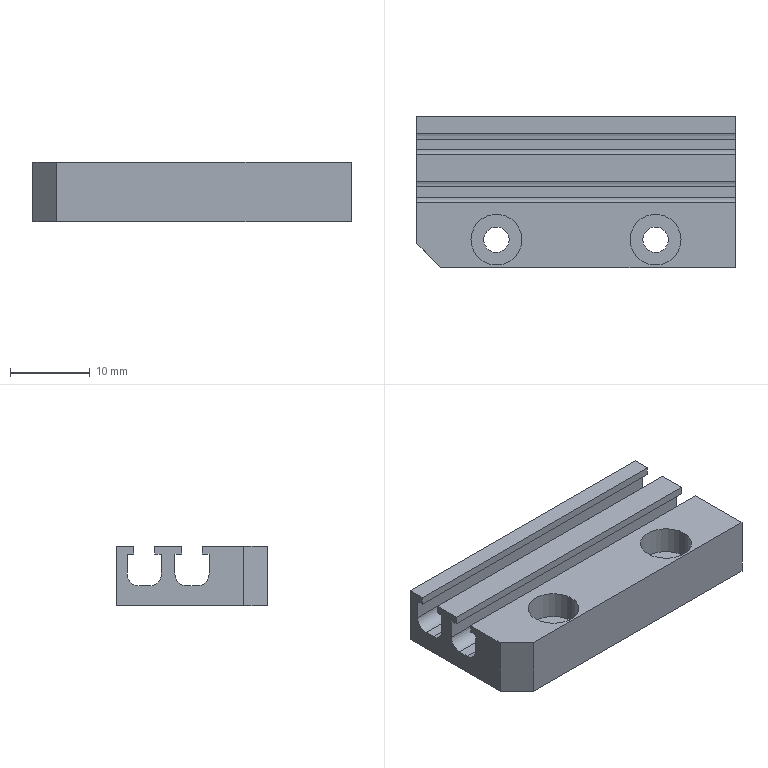Part | NX | 1 solid | 37 faces | box 40 x 19 x 7.5 mm | volume 3870 mm3 | plane 25 | cylinder 12 | commonest cylinder face diameters 3 x4 3.2 x4 6.4 x4
STEP:
#1=CARTESIAN_POINT('',(-20.,16.8,0.));
#2=VERTEX_POINT('',#1);
#3=CARTESIAN_POINT('',(-20.,19.,0.));
#4=VERTEX_POINT('',#3);
#5=CARTESIAN_POINT('',(-20.,16.8,0.));
#6=DIRECTION('',(0.,1.,0.));
#7=VECTOR('',#6,1000.);
#8=LINE('',#5,#7);
#9=EDGE_CURVE('',#2,#4,#8,.T.);
#10=ORIENTED_EDGE('',*,*,#9,.T.);
#11=CARTESIAN_POINT('',(-20.,19.,-7.5));
#12=VERTEX_POINT('',#11);
#13=CARTESIAN_POINT('',(-20.,19.,0.));
#14=DIRECTION('',(0.,0.,-1.));
#15=VECTOR('',#14,1000.);
#16=LINE('',#13,#15);
#17=EDGE_CURVE('',#4,#12,#16,.T.);
#18=ORIENTED_EDGE('',*,*,#17,.T.);
#19=CARTESIAN_POINT('',(-20.,3.,-7.5));
#20=VERTEX_POINT('',#19);
#21=CARTESIAN_POINT('',(-20.,19.,-7.5));
#22=DIRECTION('',(0.,-1.,0.));
#23=VECTOR('',#22,1000.);
#24=LINE('',#21,#23);
#25=EDGE_CURVE('',#12,#20,#24,.T.);
#26=ORIENTED_EDGE('',*,*,#25,.T.);
#27=CARTESIAN_POINT('',(-20.,3.,0.));
#28=VERTEX_POINT('',#27);
#29=CARTESIAN_POINT('',(-20.,3.,-7.5));
#30=DIRECTION('',(0.,0.,1.));
#31=VECTOR('',#30,1000.);
#32=LINE('',#29,#31);
#33=EDGE_CURVE('',#20,#28,#32,.T.);
#34=ORIENTED_EDGE('',*,*,#33,.T.);
#35=CARTESIAN_POINT('',(-20.,8.2,0.));
#36=VERTEX_POINT('',#35);
#37=CARTESIAN_POINT('',(-20.,3.,0.));
#38=DIRECTION('',(0.,1.,0.));
#39=VECTOR('',#38,1000.);
#40=LINE('',#37,#39);
#41=EDGE_CURVE('',#28,#36,#40,.T.);
#42=ORIENTED_EDGE('',*,*,#41,.T.);
#43=CARTESIAN_POINT('',(-20.,8.2,-1.));
#44=VERTEX_POINT('',#43);
#45=CARTESIAN_POINT('',(-20.,8.2,0.));
#46=DIRECTION('',(0.,0.,-1.));
#47=VECTOR('',#46,1000.);
#48=LINE('',#45,#47);
#49=EDGE_CURVE('',#36,#44,#48,.T.);
#50=ORIENTED_EDGE('',*,*,#49,.T.);
#51=CARTESIAN_POINT('',(-20.,7.35,-1.));
#52=VERTEX_POINT('',#51);
#53=CARTESIAN_POINT('',(-20.,8.2,-1.));
#54=DIRECTION('',(0.,-1.,0.));
#55=VECTOR('',#54,1000.);
#56=LINE('',#53,#55);
#57=EDGE_CURVE('',#44,#52,#56,.T.);
#58=ORIENTED_EDGE('',*,*,#57,.T.);
#59=CARTESIAN_POINT('',(-20.,7.35,-3.5));
#60=VERTEX_POINT('',#59);
#61=CARTESIAN_POINT('',(-20.,7.35,-1.));
#62=DIRECTION('',(0.,0.,-1.));
#63=VECTOR('',#62,1000.);
#64=LINE('',#61,#63);
#65=EDGE_CURVE('',#52,#60,#64,.T.);
#66=ORIENTED_EDGE('',*,*,#65,.T.);
#67=CARTESIAN_POINT('',(-20.,8.85,-5.));
#68=VERTEX_POINT('',#67);
#69=CARTESIAN_POINT('',(-20.,8.85,-3.5));
#70=DIRECTION('',(-1.,0.,0.));
#71=DIRECTION('',(0.,0.,-1.));
#72=AXIS2_PLACEMENT_3D('',#69,#70,#71);
#73=CIRCLE('',#72,1.5);
#74=EDGE_CURVE('',#68,#60,#73,.T.);
#75=ORIENTED_EDGE('',*,*,#74,.F.);
#76=CARTESIAN_POINT('',(-20.,10.15,-5.));
#77=VERTEX_POINT('',#76);
#78=CARTESIAN_POINT('',(-20.,8.85,-5.));
#79=DIRECTION('',(0.,1.,0.));
#80=VECTOR('',#79,1000.);
#81=LINE('',#78,#80);
#82=EDGE_CURVE('',#68,#77,#81,.T.);
#83=ORIENTED_EDGE('',*,*,#82,.T.);
#84=CARTESIAN_POINT('',(-20.,11.65,-3.5));
#85=VERTEX_POINT('',#84);
#86=CARTESIAN_POINT('',(-20.,10.15,-3.5));
#87=DIRECTION('',(-1.,0.,0.));
#88=DIRECTION('',(0.,1.,0.));
#89=AXIS2_PLACEMENT_3D('',#86,#87,#88);
#90=CIRCLE('',#89,1.5);
#91=EDGE_CURVE('',#85,#77,#90,.T.);
#92=ORIENTED_EDGE('',*,*,#91,.F.);
#93=CARTESIAN_POINT('',(-20.,11.65,-1.));
#94=VERTEX_POINT('',#93);
#95=CARTESIAN_POINT('',(-20.,11.65,-3.5));
#96=DIRECTION('',(0.,0.,1.));
#97=VECTOR('',#96,1000.);
#98=LINE('',#95,#97);
#99=EDGE_CURVE('',#85,#94,#98,.T.);
#100=ORIENTED_EDGE('',*,*,#99,.T.);
#101=CARTESIAN_POINT('',(-20.,10.8,-1.));
#102=VERTEX_POINT('',#101);
#103=CARTESIAN_POINT('',(-20.,11.65,-1.));
#104=DIRECTION('',(0.,-1.,0.));
#105=VECTOR('',#104,1000.);
#106=LINE('',#103,#105);
#107=EDGE_CURVE('',#94,#102,#106,.T.);
#108=ORIENTED_EDGE('',*,*,#107,.T.);
#109=CARTESIAN_POINT('',(-20.,10.8,0.));
#110=VERTEX_POINT('',#109);
#111=CARTESIAN_POINT('',(-20.,10.8,-1.));
#112=DIRECTION('',(0.,0.,1.));
#113=VECTOR('',#112,1000.);
#114=LINE('',#111,#113);
#115=EDGE_CURVE('',#102,#110,#114,.T.);
#116=ORIENTED_EDGE('',*,*,#115,.T.);
#117=CARTESIAN_POINT('',(-20.,14.2,0.));
#118=VERTEX_POINT('',#117);
#119=CARTESIAN_POINT('',(-20.,10.8,0.));
#120=DIRECTION('',(0.,1.,0.));
#121=VECTOR('',#120,1000.);
#122=LINE('',#119,#121);
#123=EDGE_CURVE('',#110,#118,#122,.T.);
#124=ORIENTED_EDGE('',*,*,#123,.T.);
#125=CARTESIAN_POINT('',(-20.,14.2,-1.));
#126=VERTEX_POINT('',#125);
#127=CARTESIAN_POINT('',(-20.,14.2,0.));
#128=DIRECTION('',(0.,0.,-1.));
#129=VECTOR('',#128,1000.);
#130=LINE('',#127,#129);
#131=EDGE_CURVE('',#118,#126,#130,.T.);
#132=ORIENTED_EDGE('',*,*,#131,.T.);
#133=CARTESIAN_POINT('',(-20.,13.35,-1.));
#134=VERTEX_POINT('',#133);
#135=CARTESIAN_POINT('',(-20.,14.2,-1.));
#136=DIRECTION('',(0.,-1.,0.));
#137=VECTOR('',#136,1000.);
#138=LINE('',#135,#137);
#139=EDGE_CURVE('',#126,#134,#138,.T.);
#140=ORIENTED_EDGE('',*,*,#139,.T.);
#141=CARTESIAN_POINT('',(-20.,13.35,-3.5));
#142=VERTEX_POINT('',#141);
#143=CARTESIAN_POINT('',(-20.,13.35,-1.));
#144=DIRECTION('',(0.,0.,-1.));
#145=VECTOR('',#144,1000.);
#146=LINE('',#143,#145);
#147=EDGE_CURVE('',#134,#142,#146,.T.);
#148=ORIENTED_EDGE('',*,*,#147,.T.);
#149=CARTESIAN_POINT('',(-20.,14.85,-5.));
#150=VERTEX_POINT('',#149);
#151=CARTESIAN_POINT('',(-20.,14.85,-3.5));
#152=DIRECTION('',(-1.,0.,0.));
#153=DIRECTION('',(0.,0.,-1.));
#154=AXIS2_PLACEMENT_3D('',#151,#152,#153);
#155=CIRCLE('',#154,1.5);
#156=EDGE_CURVE('',#150,#142,#155,.T.);
#157=ORIENTED_EDGE('',*,*,#156,.F.);
#158=CARTESIAN_POINT('',(-20.,16.15,-5.));
#159=VERTEX_POINT('',#158);
#160=CARTESIAN_POINT('',(-20.,14.85,-5.));
#161=DIRECTION('',(0.,1.,0.));
#162=VECTOR('',#161,1000.);
#163=LINE('',#160,#162);
#164=EDGE_CURVE('',#150,#159,#163,.T.);
#165=ORIENTED_EDGE('',*,*,#164,.T.);
#166=CARTESIAN_POINT('',(-20.,17.65,-3.5));
#167=VERTEX_POINT('',#166);
#168=CARTESIAN_POINT('',(-20.,16.15,-3.5));
#169=DIRECTION('',(-1.,0.,0.));
#170=DIRECTION('',(0.,1.,0.));
#171=AXIS2_PLACEMENT_3D('',#168,#169,#170);
#172=CIRCLE('',#171,1.5);
#173=EDGE_CURVE('',#167,#159,#172,.T.);
#174=ORIENTED_EDGE('',*,*,#173,.F.);
#175=CARTESIAN_POINT('',(-20.,17.65,-1.));
#176=VERTEX_POINT('',#175);
#177=CARTESIAN_POINT('',(-20.,17.65,-3.5));
#178=DIRECTION('',(0.,0.,1.));
#179=VECTOR('',#178,1000.);
#180=LINE('',#177,#179);
#181=EDGE_CURVE('',#167,#176,#180,.T.);
#182=ORIENTED_EDGE('',*,*,#181,.T.);
#183=CARTESIAN_POINT('',(-20.,16.8,-1.));
#184=VERTEX_POINT('',#183);
#185=CARTESIAN_POINT('',(-20.,17.65,-1.));
#186=DIRECTION('',(0.,-1.,0.));
#187=VECTOR('',#186,1000.);
#188=LINE('',#185,#187);
#189=EDGE_CURVE('',#176,#184,#188,.T.);
#190=ORIENTED_EDGE('',*,*,#189,.T.);
#191=CARTESIAN_POINT('',(-20.,16.8,-1.));
#192=DIRECTION('',(0.,0.,1.));
#193=VECTOR('',#192,1000.);
#194=LINE('',#191,#193);
#195=EDGE_CURVE('',#184,#2,#194,.T.);
#196=ORIENTED_EDGE('',*,*,#195,.T.);
#197=EDGE_LOOP('',(#10,#18,#26,#34,#42,#50,#58,#66,#75,#83,#92,#100,#108,#116,#124,#132,#140,#148,#157,#165,#174,#182,#190,#196));
#198=FACE_BOUND('',#197,.T.);
#199=CARTESIAN_POINT('',(-20.,0.,0.));
#200=DIRECTION('',(1.,0.,0.));
#201=DIRECTION('',(0.,1.,0.));
#202=AXIS2_PLACEMENT_3D('',#199,#200,#201);
#203=PLANE('',#202);
#204=ADVANCED_FACE('',(#198),#203,.F.);
#205=ORIENTED_EDGE('',*,*,#9,.F.);
#206=CARTESIAN_POINT('',(20.,16.8,0.));
#207=VERTEX_POINT('',#206);
#208=CARTESIAN_POINT('',(20.,16.8,0.));
#209=DIRECTION('',(-1.,0.,0.));
#210=VECTOR('',#209,1000.);
#211=LINE('',#208,#210);
#212=EDGE_CURVE('',#207,#2,#211,.T.);
#213=ORIENTED_EDGE('',*,*,#212,.F.);
#214=CARTESIAN_POINT('',(20.,19.,0.));
#215=VERTEX_POINT('',#214);
#216=CARTESIAN_POINT('',(20.,16.8,0.));
#217=DIRECTION('',(0.,1.,0.));
#218=VECTOR('',#217,1000.);
#219=LINE('',#216,#218);
#220=EDGE_CURVE('',#207,#215,#219,.T.);
#221=ORIENTED_EDGE('',*,*,#220,.T.);
#222=CARTESIAN_POINT('',(20.,19.,0.));
#223=DIRECTION('',(-1.,0.,0.));
#224=VECTOR('',#223,1000.);
#225=LINE('',#222,#224);
#226=EDGE_CURVE('',#215,#4,#225,.T.);
#227=ORIENTED_EDGE('',*,*,#226,.T.);
#228=EDGE_LOOP('',(#205,#213,#221,#227));
#229=FACE_BOUND('',#228,.T.);
#230=CARTESIAN_POINT('',(-20.,19.,0.));
#231=DIRECTION('',(0.,0.,1.));
#232=DIRECTION('',(1.,0.,0.));
#233=AXIS2_PLACEMENT_3D('',#230,#231,#232);
#234=PLANE('',#233);
#235=ADVANCED_FACE('',(#229),#234,.T.);
#236=ORIENTED_EDGE('',*,*,#17,.F.);
#237=ORIENTED_EDGE('',*,*,#226,.F.);
#238=CARTESIAN_POINT('',(20.,19.,-7.5));
#239=VERTEX_POINT('',#238);
#240=CARTESIAN_POINT('',(20.,19.,0.));
#241=DIRECTION('',(0.,0.,-1.));
#242=VECTOR('',#241,1000.);
#243=LINE('',#240,#242);
#244=EDGE_CURVE('',#215,#239,#243,.T.);
#245=ORIENTED_EDGE('',*,*,#244,.T.);
#246=CARTESIAN_POINT('',(20.,19.,-7.5));
#247=DIRECTION('',(-1.,0.,0.));
#248=VECTOR('',#247,1000.);
#249=LINE('',#246,#248);
#250=EDGE_CURVE('',#239,#12,#249,.T.);
#251=ORIENTED_EDGE('',*,*,#250,.T.);
#252=EDGE_LOOP('',(#236,#237,#245,#251));
#253=FACE_BOUND('',#252,.T.);
#254=CARTESIAN_POINT('',(-20.,19.,-7.5));
#255=DIRECTION('',(0.,1.,0.));
#256=DIRECTION('',(1.,0.,0.));
#257=AXIS2_PLACEMENT_3D('',#254,#255,#256);
#258=PLANE('',#257);
#259=ADVANCED_FACE('',(#253),#258,.T.);
#260=ORIENTED_EDGE('',*,*,#25,.F.);
#261=ORIENTED_EDGE('',*,*,#250,.F.);
#262=CARTESIAN_POINT('',(20.,0.,-7.5));
#263=VERTEX_POINT('',#262);
#264=CARTESIAN_POINT('',(20.,19.,-7.5));
#265=DIRECTION('',(0.,-1.,0.));
#266=VECTOR('',#265,1000.);
#267=LINE('',#264,#266);
#268=EDGE_CURVE('',#239,#263,#267,.T.);
#269=ORIENTED_EDGE('',*,*,#268,.T.);
#270=CARTESIAN_POINT('',(-17.,0.,-7.5));
#271=VERTEX_POINT('',#270);
#272=CARTESIAN_POINT('',(20.,0.,-7.5));
#273=DIRECTION('',(-1.,0.,0.));
#274=VECTOR('',#273,1000.);
#275=LINE('',#272,#274);
#276=EDGE_CURVE('',#263,#271,#275,.T.);
#277=ORIENTED_EDGE('',*,*,#276,.T.);
#278=CARTESIAN_POINT('',(-20.,3.,-7.5));
#279=DIRECTION('',(0.7071,-0.7071,0.));
#280=VECTOR('',#279,1000.);
#281=LINE('',#278,#280);
#282=EDGE_CURVE('',#20,#271,#281,.T.);
#283=ORIENTED_EDGE('',*,*,#282,.F.);
#284=EDGE_LOOP('',(#260,#261,#269,#277,#283));
#285=FACE_BOUND('',#284,.T.);
#286=CARTESIAN_POINT('',(-8.4,3.5,-7.5));
#287=VERTEX_POINT('',#286);
#288=CARTESIAN_POINT('',(-11.6,3.5,-7.5));
#289=VERTEX_POINT('',#288);
#290=CARTESIAN_POINT('',(-10.,3.5,-7.5));
#291=DIRECTION('',(0.,0.,-1.));
#292=DIRECTION('',(-1.,0.,0.));
#293=AXIS2_PLACEMENT_3D('',#290,#291,#292);
#294=CIRCLE('',#293,1.6);
#295=EDGE_CURVE('',#287,#289,#294,.T.);
#296=ORIENTED_EDGE('',*,*,#295,.F.);
#297=CARTESIAN_POINT('',(-10.,3.5,-7.5));
#298=DIRECTION('',(0.,0.,-1.));
#299=DIRECTION('',(-1.,0.,0.));
#300=AXIS2_PLACEMENT_3D('',#297,#298,#299);
#301=CIRCLE('',#300,1.6);
#302=EDGE_CURVE('',#289,#287,#301,.T.);
#303=ORIENTED_EDGE('',*,*,#302,.F.);
#304=EDGE_LOOP('',(#296,#303));
#305=FACE_BOUND('',#304,.T.);
#306=CARTESIAN_POINT('',(11.6,3.5,-7.5));
#307=VERTEX_POINT('',#306);
#308=CARTESIAN_POINT('',(8.4,3.5,-7.5));
#309=VERTEX_POINT('',#308);
#310=CARTESIAN_POINT('',(10.,3.5,-7.5));
#311=DIRECTION('',(0.,0.,-1.));
#312=DIRECTION('',(-1.,0.,0.));
#313=AXIS2_PLACEMENT_3D('',#310,#311,#312);
#314=CIRCLE('',#313,1.6);
#315=EDGE_CURVE('',#307,#309,#314,.T.);
#316=ORIENTED_EDGE('',*,*,#315,.F.);
#317=CARTESIAN_POINT('',(10.,3.5,-7.5));
#318=DIRECTION('',(0.,0.,-1.));
#319=DIRECTION('',(-1.,0.,0.));
#320=AXIS2_PLACEMENT_3D('',#317,#318,#319);
#321=CIRCLE('',#320,1.6);
#322=EDGE_CURVE('',#309,#307,#321,.T.);
#323=ORIENTED_EDGE('',*,*,#322,.F.);
#324=EDGE_LOOP('',(#316,#323));
#325=FACE_BOUND('',#324,.T.);
#326=CARTESIAN_POINT('',(-20.,0.,-7.5));
#327=DIRECTION('',(0.,0.,-1.));
#328=DIRECTION('',(0.,-1.,0.));
#329=AXIS2_PLACEMENT_3D('',#326,#327,#328);
#330=PLANE('',#329);
#331=ADVANCED_FACE('',(#285,#305,#325),#330,.T.);
#332=ORIENTED_EDGE('',*,*,#33,.F.);
#333=ORIENTED_EDGE('',*,*,#282,.T.);
#334=CARTESIAN_POINT('',(-17.,0.,0.));
#335=VERTEX_POINT('',#334);
#336=CARTESIAN_POINT('',(-17.,0.,-7.5));
#337=DIRECTION('',(0.,0.,1.));
#338=VECTOR('',#337,1000.);
#339=LINE('',#336,#338);
#340=EDGE_CURVE('',#271,#335,#339,.T.);
#341=ORIENTED_EDGE('',*,*,#340,.T.);
#342=CARTESIAN_POINT('',(-17.,0.,0.));
#343=DIRECTION('',(-0.7071,0.7071,0.));
#344=VECTOR('',#343,1000.);
#345=LINE('',#342,#344);
#346=EDGE_CURVE('',#335,#28,#345,.T.);
#347=ORIENTED_EDGE('',*,*,#346,.T.);
#348=EDGE_LOOP('',(#332,#333,#341,#347));
#349=FACE_BOUND('',#348,.T.);
#350=CARTESIAN_POINT('',(-20.,3.,0.));
#351=DIRECTION('',(-0.7071,-0.7071,0.));
#352=DIRECTION('',(-0.7071,0.7071,0.));
#353=AXIS2_PLACEMENT_3D('',#350,#351,#352);
#354=PLANE('',#353);
#355=ADVANCED_FACE('',(#349),#354,.T.);
#356=ORIENTED_EDGE('',*,*,#41,.F.);
#357=ORIENTED_EDGE('',*,*,#346,.F.);
#358=CARTESIAN_POINT('',(20.,0.,0.));
#359=VERTEX_POINT('',#358);
#360=CARTESIAN_POINT('',(20.,0.,0.));
#361=DIRECTION('',(-1.,0.,0.));
#362=VECTOR('',#361,1000.);
#363=LINE('',#360,#362);
#364=EDGE_CURVE('',#359,#335,#363,.T.);
#365=ORIENTED_EDGE('',*,*,#364,.F.);
#366=CARTESIAN_POINT('',(20.,8.2,0.));
#367=VERTEX_POINT('',#366);
#368=CARTESIAN_POINT('',(20.,0.,0.));
#369=DIRECTION('',(0.,1.,0.));
#370=VECTOR('',#369,1000.);
#371=LINE('',#368,#370);
#372=EDGE_CURVE('',#359,#367,#371,.T.);
#373=ORIENTED_EDGE('',*,*,#372,.T.);
#374=CARTESIAN_POINT('',(20.,8.2,0.));
#375=DIRECTION('',(-1.,0.,0.));
#376=VECTOR('',#375,1000.);
#377=LINE('',#374,#376);
#378=EDGE_CURVE('',#367,#36,#377,.T.);
#379=ORIENTED_EDGE('',*,*,#378,.T.);
#380=EDGE_LOOP('',(#356,#357,#365,#373,#379));
#381=FACE_BOUND('',#380,.T.);
#382=CARTESIAN_POINT('',(-13.2,3.5,0.));
#383=VERTEX_POINT('',#382);
#384=CARTESIAN_POINT('',(-6.8,3.5,0.));
#385=VERTEX_POINT('',#384);
#386=CARTESIAN_POINT('',(-10.,3.5,0.));
#387=DIRECTION('',(0.,0.,1.));
#388=DIRECTION('',(1.,0.,0.));
#389=AXIS2_PLACEMENT_3D('',#386,#387,#388);
#390=CIRCLE('',#389,3.2);
#391=EDGE_CURVE('',#383,#385,#390,.T.);
#392=ORIENTED_EDGE('',*,*,#391,.F.);
#393=CARTESIAN_POINT('',(-10.,3.5,0.));
#394=DIRECTION('',(0.,0.,1.));
#395=DIRECTION('',(1.,0.,0.));
#396=AXIS2_PLACEMENT_3D('',#393,#394,#395);
#397=CIRCLE('',#396,3.2);
#398=EDGE_CURVE('',#385,#383,#397,.T.);
#399=ORIENTED_EDGE('',*,*,#398,.F.);
#400=EDGE_LOOP('',(#392,#399));
#401=FACE_BOUND('',#400,.T.);
#402=CARTESIAN_POINT('',(13.2,3.5,0.));
#403=VERTEX_POINT('',#402);
#404=CARTESIAN_POINT('',(6.8,3.5,0.));
#405=VERTEX_POINT('',#404);
#406=CARTESIAN_POINT('',(10.,3.5,0.));
#407=DIRECTION('',(0.,0.,1.));
#408=DIRECTION('',(1.,0.,0.));
#409=AXIS2_PLACEMENT_3D('',#406,#407,#408);
#410=CIRCLE('',#409,3.2);
#411=EDGE_CURVE('',#403,#405,#410,.T.);
#412=ORIENTED_EDGE('',*,*,#411,.F.);
#413=CARTESIAN_POINT('',(10.,3.5,0.));
#414=DIRECTION('',(0.,0.,1.));
#415=DIRECTION('',(1.,0.,0.));
#416=AXIS2_PLACEMENT_3D('',#413,#414,#415);
#417=CIRCLE('',#416,3.2);
#418=EDGE_CURVE('',#405,#403,#417,.T.);
#419=ORIENTED_EDGE('',*,*,#418,.F.);
#420=EDGE_LOOP('',(#412,#419));
#421=FACE_BOUND('',#420,.T.);
#422=CARTESIAN_POINT('',(-20.,8.2,0.));
#423=DIRECTION('',(0.,0.,1.));
#424=DIRECTION('',(1.,0.,0.));
#425=AXIS2_PLACEMENT_3D('',#422,#423,#424);
#426=PLANE('',#425);
#427=ADVANCED_FACE('',(#381,#401,#421),#426,.T.);
#428=ORIENTED_EDGE('',*,*,#49,.F.);
#429=ORIENTED_EDGE('',*,*,#378,.F.);
#430=CARTESIAN_POINT('',(20.,8.2,-1.));
#431=VERTEX_POINT('',#430);
#432=CARTESIAN_POINT('',(20.,8.2,0.));
#433=DIRECTION('',(0.,0.,-1.));
#434=VECTOR('',#433,1000.);
#435=LINE('',#432,#434);
#436=EDGE_CURVE('',#367,#431,#435,.T.);
#437=ORIENTED_EDGE('',*,*,#436,.T.);
#438=CARTESIAN_POINT('',(20.,8.2,-1.));
#439=DIRECTION('',(-1.,0.,0.));
#440=VECTOR('',#439,1000.);
#441=LINE('',#438,#440);
#442=EDGE_CURVE('',#431,#44,#441,.T.);
#443=ORIENTED_EDGE('',*,*,#442,.T.);
#444=EDGE_LOOP('',(#428,#429,#437,#443));
#445=FACE_BOUND('',#444,.T.);
#446=CARTESIAN_POINT('',(-20.,8.2,-1.));
#447=DIRECTION('',(0.,1.,0.));
#448=DIRECTION('',(1.,0.,0.));
#449=AXIS2_PLACEMENT_3D('',#446,#447,#448);
#450=PLANE('',#449);
#451=ADVANCED_FACE('',(#445),#450,.T.);
#452=ORIENTED_EDGE('',*,*,#57,.F.);
#453=ORIENTED_EDGE('',*,*,#442,.F.);
#454=CARTESIAN_POINT('',(20.,7.35,-1.));
#455=VERTEX_POINT('',#454);
#456=CARTESIAN_POINT('',(20.,8.2,-1.));
#457=DIRECTION('',(0.,-1.,0.));
#458=VECTOR('',#457,1000.);
#459=LINE('',#456,#458);
#460=EDGE_CURVE('',#431,#455,#459,.T.);
#461=ORIENTED_EDGE('',*,*,#460,.T.);
#462=CARTESIAN_POINT('',(20.,7.35,-1.));
#463=DIRECTION('',(-1.,0.,0.));
#464=VECTOR('',#463,1000.);
#465=LINE('',#462,#464);
#466=EDGE_CURVE('',#455,#52,#465,.T.);
#467=ORIENTED_EDGE('',*,*,#466,.T.);
#468=EDGE_LOOP('',(#452,#453,#461,#467));
#469=FACE_BOUND('',#468,.T.);
#470=CARTESIAN_POINT('',(-20.,7.35,-1.));
#471=DIRECTION('',(0.,0.,-1.));
#472=DIRECTION('',(0.,-1.,0.));
#473=AXIS2_PLACEMENT_3D('',#470,#471,#472);
#474=PLANE('',#473);
#475=ADVANCED_FACE('',(#469),#474,.T.);
#476=ORIENTED_EDGE('',*,*,#65,.F.);
#477=ORIENTED_EDGE('',*,*,#466,.F.);
#478=CARTESIAN_POINT('',(20.,7.35,-3.5));
#479=VERTEX_POINT('',#478);
#480=CARTESIAN_POINT('',(20.,7.35,-1.));
#481=DIRECTION('',(0.,0.,-1.));
#482=VECTOR('',#481,1000.);
#483=LINE('',#480,#482);
#484=EDGE_CURVE('',#455,#479,#483,.T.);
#485=ORIENTED_EDGE('',*,*,#484,.T.);
#486=CARTESIAN_POINT('',(20.,7.35,-3.5));
#487=DIRECTION('',(-1.,0.,0.));
#488=VECTOR('',#487,1000.);
#489=LINE('',#486,#488);
#490=EDGE_CURVE('',#479,#60,#489,.T.);
#491=ORIENTED_EDGE('',*,*,#490,.T.);
#492=EDGE_LOOP('',(#476,#477,#485,#491));
#493=FACE_BOUND('',#492,.T.);
#494=CARTESIAN_POINT('',(-20.,7.35,-3.5));
#495=DIRECTION('',(0.,1.,0.));
#496=DIRECTION('',(1.,0.,0.));
#497=AXIS2_PLACEMENT_3D('',#494,#495,#496);
#498=PLANE('',#497);
#499=ADVANCED_FACE('',(#493),#498,.T.);
#500=ORIENTED_EDGE('',*,*,#74,.T.);
#501=ORIENTED_EDGE('',*,*,#490,.F.);
#502=CARTESIAN_POINT('',(20.,8.85,-5.));
#503=VERTEX_POINT('',#502);
#504=CARTESIAN_POINT('',(20.,8.85,-3.5));
#505=DIRECTION('',(1.,0.,0.));
#506=DIRECTION('',(0.,-1.,0.));
#507=AXIS2_PLACEMENT_3D('',#504,#505,#506);
#508=CIRCLE('',#507,1.5);
#509=EDGE_CURVE('',#479,#503,#508,.T.);
#510=ORIENTED_EDGE('',*,*,#509,.T.);
#511=CARTESIAN_POINT('',(-20.,8.85,-5.));
#512=DIRECTION('',(1.,0.,0.));
#513=VECTOR('',#512,1000.);
#514=LINE('',#511,#513);
#515=EDGE_CURVE('',#68,#503,#514,.T.);
#516=ORIENTED_EDGE('',*,*,#515,.F.);
#517=EDGE_LOOP('',(#500,#501,#510,#516));
#518=FACE_BOUND('',#517,.T.);
#519=CARTESIAN_POINT('',(-20.,8.85,-3.5));
#520=DIRECTION('',(1.,0.,0.));
#521=DIRECTION('',(0.,0.,-1.));
#522=AXIS2_PLACEMENT_3D('',#519,#520,#521);
#523=CYLINDRICAL_SURFACE('',#522,1.5);
#524=ADVANCED_FACE('',(#518),#523,.F.);
#525=ORIENTED_EDGE('',*,*,#82,.F.);
#526=ORIENTED_EDGE('',*,*,#515,.T.);
#527=CARTESIAN_POINT('',(20.,10.15,-5.));
#528=VERTEX_POINT('',#527);
#529=CARTESIAN_POINT('',(20.,8.85,-5.));
#530=DIRECTION('',(0.,1.,0.));
#531=VECTOR('',#530,1000.);
#532=LINE('',#529,#531);
#533=EDGE_CURVE('',#503,#528,#532,.T.);
#534=ORIENTED_EDGE('',*,*,#533,.T.);
#535=CARTESIAN_POINT('',(-20.,10.15,-5.));
#536=DIRECTION('',(1.,0.,0.));
#537=VECTOR('',#536,1000.);
#538=LINE('',#535,#537);
#539=EDGE_CURVE('',#77,#528,#538,.T.);
#540=ORIENTED_EDGE('',*,*,#539,.F.);
#541=EDGE_LOOP('',(#525,#526,#534,#540));
#542=FACE_BOUND('',#541,.T.);
#543=CARTESIAN_POINT('',(-20.,10.15,-5.));
#544=DIRECTION('',(0.,0.,1.));
#545=DIRECTION('',(1.,0.,0.));
#546=AXIS2_PLACEMENT_3D('',#543,#544,#545);
#547=PLANE('',#546);
#548=ADVANCED_FACE('',(#542),#547,.T.);
#549=ORIENTED_EDGE('',*,*,#91,.T.);
#550=ORIENTED_EDGE('',*,*,#539,.T.);
#551=CARTESIAN_POINT('',(20.,11.65,-3.5));
#552=VERTEX_POINT('',#551);
#553=CARTESIAN_POINT('',(20.,10.15,-3.5));
#554=DIRECTION('',(1.,0.,0.));
#555=DIRECTION('',(0.,0.,-1.));
#556=AXIS2_PLACEMENT_3D('',#553,#554,#555);
#557=CIRCLE('',#556,1.5);
#558=EDGE_CURVE('',#528,#552,#557,.T.);
#559=ORIENTED_EDGE('',*,*,#558,.T.);
#560=CARTESIAN_POINT('',(-20.,11.65,-3.5));
#561=DIRECTION('',(1.,0.,0.));
#562=VECTOR('',#561,1000.);
#563=LINE('',#560,#562);
#564=EDGE_CURVE('',#85,#552,#563,.T.);
#565=ORIENTED_EDGE('',*,*,#564,.F.);
#566=EDGE_LOOP('',(#549,#550,#559,#565));
#567=FACE_BOUND('',#566,.T.);
#568=CARTESIAN_POINT('',(-20.,10.15,-3.5));
#569=DIRECTION('',(1.,0.,0.));
#570=DIRECTION('',(0.,0.,-1.));
#571=AXIS2_PLACEMENT_3D('',#568,#569,#570);
#572=CYLINDRICAL_SURFACE('',#571,1.5);
#573=ADVANCED_FACE('',(#567),#572,.F.);
#574=ORIENTED_EDGE('',*,*,#99,.F.);
#575=ORIENTED_EDGE('',*,*,#564,.T.);
#576=CARTESIAN_POINT('',(20.,11.65,-1.));
#577=VERTEX_POINT('',#576);
#578=CARTESIAN_POINT('',(20.,11.65,-3.5));
#579=DIRECTION('',(0.,0.,1.));
#580=VECTOR('',#579,1000.);
#581=LINE('',#578,#580);
#582=EDGE_CURVE('',#552,#577,#581,.T.);
#583=ORIENTED_EDGE('',*,*,#582,.T.);
#584=CARTESIAN_POINT('',(20.,11.65,-1.));
#585=DIRECTION('',(-1.,0.,0.));
#586=VECTOR('',#585,1000.);
#587=LINE('',#584,#586);
#588=EDGE_CURVE('',#577,#94,#587,.T.);
#589=ORIENTED_EDGE('',*,*,#588,.T.);
#590=EDGE_LOOP('',(#574,#575,#583,#589));
#591=FACE_BOUND('',#590,.T.);
#592=CARTESIAN_POINT('',(-20.,11.65,-1.));
#593=DIRECTION('',(0.,-1.,0.));
#594=DIRECTION('',(0.,0.,-1.));
#595=AXIS2_PLACEMENT_3D('',#592,#593,#594);
#596=PLANE('',#595);
#597=ADVANCED_FACE('',(#591),#596,.T.);
#598=ORIENTED_EDGE('',*,*,#107,.F.);
#599=ORIENTED_EDGE('',*,*,#588,.F.);
#600=CARTESIAN_POINT('',(20.,10.8,-1.));
#601=VERTEX_POINT('',#600);
#602=CARTESIAN_POINT('',(20.,11.65,-1.));
#603=DIRECTION('',(0.,-1.,0.));
#604=VECTOR('',#603,1000.);
#605=LINE('',#602,#604);
#606=EDGE_CURVE('',#577,#601,#605,.T.);
#607=ORIENTED_EDGE('',*,*,#606,.T.);
#608=CARTESIAN_POINT('',(20.,10.8,-1.));
#609=DIRECTION('',(-1.,0.,0.));
#610=VECTOR('',#609,1000.);
#611=LINE('',#608,#610);
#612=EDGE_CURVE('',#601,#102,#611,.T.);
#613=ORIENTED_EDGE('',*,*,#612,.T.);
#614=EDGE_LOOP('',(#598,#599,#607,#613));
#615=FACE_BOUND('',#614,.T.);
#616=CARTESIAN_POINT('',(-20.,10.8,-1.));
#617=DIRECTION('',(0.,0.,-1.));
#618=DIRECTION('',(0.,-1.,0.));
#619=AXIS2_PLACEMENT_3D('',#616,#617,#618);
#620=PLANE('',#619);
#621=ADVANCED_FACE('',(#615),#620,.T.);
#622=ORIENTED_EDGE('',*,*,#115,.F.);
#623=ORIENTED_EDGE('',*,*,#612,.F.);
#624=CARTESIAN_POINT('',(20.,10.8,0.));
#625=VERTEX_POINT('',#624);
#626=CARTESIAN_POINT('',(20.,10.8,-1.));
#627=DIRECTION('',(0.,0.,1.));
#628=VECTOR('',#627,1000.);
#629=LINE('',#626,#628);
#630=EDGE_CURVE('',#601,#625,#629,.T.);
#631=ORIENTED_EDGE('',*,*,#630,.T.);
#632=CARTESIAN_POINT('',(20.,10.8,0.));
#633=DIRECTION('',(-1.,0.,0.));
#634=VECTOR('',#633,1000.);
#635=LINE('',#632,#634);
#636=EDGE_CURVE('',#625,#110,#635,.T.);
#637=ORIENTED_EDGE('',*,*,#636,.T.);
#638=EDGE_LOOP('',(#622,#623,#631,#637));
#639=FACE_BOUND('',#638,.T.);
#640=CARTESIAN_POINT('',(-20.,10.8,0.));
#641=DIRECTION('',(0.,-1.,0.));
#642=DIRECTION('',(0.,0.,-1.));
#643=AXIS2_PLACEMENT_3D('',#640,#641,#642);
#644=PLANE('',#643);
#645=ADVANCED_FACE('',(#639),#644,.T.);
#646=ORIENTED_EDGE('',*,*,#123,.F.);
#647=ORIENTED_EDGE('',*,*,#636,.F.);
#648=CARTESIAN_POINT('',(20.,14.2,0.));
#649=VERTEX_POINT('',#648);
#650=CARTESIAN_POINT('',(20.,10.8,0.));
#651=DIRECTION('',(0.,1.,0.));
#652=VECTOR('',#651,1000.);
#653=LINE('',#650,#652);
#654=EDGE_CURVE('',#625,#649,#653,.T.);
#655=ORIENTED_EDGE('',*,*,#654,.T.);
#656=CARTESIAN_POINT('',(20.,14.2,0.));
#657=DIRECTION('',(-1.,0.,0.));
#658=VECTOR('',#657,1000.);
#659=LINE('',#656,#658);
#660=EDGE_CURVE('',#649,#118,#659,.T.);
#661=ORIENTED_EDGE('',*,*,#660,.T.);
#662=EDGE_LOOP('',(#646,#647,#655,#661));
#663=FACE_BOUND('',#662,.T.);
#664=CARTESIAN_POINT('',(-20.,14.2,0.));
#665=DIRECTION('',(0.,0.,1.));
#666=DIRECTION('',(1.,0.,0.));
#667=AXIS2_PLACEMENT_3D('',#664,#665,#666);
#668=PLANE('',#667);
#669=ADVANCED_FACE('',(#663),#668,.T.);
#670=ORIENTED_EDGE('',*,*,#131,.F.);
#671=ORIENTED_EDGE('',*,*,#660,.F.);
#672=CARTESIAN_POINT('',(20.,14.2,-1.));
#673=VERTEX_POINT('',#672);
#674=CARTESIAN_POINT('',(20.,14.2,0.));
#675=DIRECTION('',(0.,0.,-1.));
#676=VECTOR('',#675,1000.);
#677=LINE('',#674,#676);
#678=EDGE_CURVE('',#649,#673,#677,.T.);
#679=ORIENTED_EDGE('',*,*,#678,.T.);
#680=CARTESIAN_POINT('',(20.,14.2,-1.));
#681=DIRECTION('',(-1.,0.,0.));
#682=VECTOR('',#681,1000.);
#683=LINE('',#680,#682);
#684=EDGE_CURVE('',#673,#126,#683,.T.);
#685=ORIENTED_EDGE('',*,*,#684,.T.);
#686=EDGE_LOOP('',(#670,#671,#679,#685));
#687=FACE_BOUND('',#686,.T.);
#688=CARTESIAN_POINT('',(-20.,14.2,-1.));
#689=DIRECTION('',(0.,1.,0.));
#690=DIRECTION('',(1.,0.,0.));
#691=AXIS2_PLACEMENT_3D('',#688,#689,#690);
#692=PLANE('',#691);
#693=ADVANCED_FACE('',(#687),#692,.T.);
#694=ORIENTED_EDGE('',*,*,#139,.F.);
#695=ORIENTED_EDGE('',*,*,#684,.F.);
#696=CARTESIAN_POINT('',(20.,13.35,-1.));
#697=VERTEX_POINT('',#696);
#698=CARTESIAN_POINT('',(20.,14.2,-1.));
#699=DIRECTION('',(0.,-1.,0.));
#700=VECTOR('',#699,1000.);
#701=LINE('',#698,#700);
#702=EDGE_CURVE('',#673,#697,#701,.T.);
#703=ORIENTED_EDGE('',*,*,#702,.T.);
#704=CARTESIAN_POINT('',(20.,13.35,-1.));
#705=DIRECTION('',(-1.,0.,0.));
#706=VECTOR('',#705,1000.);
#707=LINE('',#704,#706);
#708=EDGE_CURVE('',#697,#134,#707,.T.);
#709=ORIENTED_EDGE('',*,*,#708,.T.);
#710=EDGE_LOOP('',(#694,#695,#703,#709));
#711=FACE_BOUND('',#710,.T.);
#712=CARTESIAN_POINT('',(-20.,13.35,-1.));
#713=DIRECTION('',(0.,0.,-1.));
#714=DIRECTION('',(0.,-1.,0.));
#715=AXIS2_PLACEMENT_3D('',#712,#713,#714);
#716=PLANE('',#715);
#717=ADVANCED_FACE('',(#711),#716,.T.);
#718=ORIENTED_EDGE('',*,*,#147,.F.);
#719=ORIENTED_EDGE('',*,*,#708,.F.);
#720=CARTESIAN_POINT('',(20.,13.35,-3.5));
#721=VERTEX_POINT('',#720);
#722=CARTESIAN_POINT('',(20.,13.35,-1.));
#723=DIRECTION('',(0.,0.,-1.));
#724=VECTOR('',#723,1000.);
#725=LINE('',#722,#724);
#726=EDGE_CURVE('',#697,#721,#725,.T.);
#727=ORIENTED_EDGE('',*,*,#726,.T.);
#728=CARTESIAN_POINT('',(20.,13.35,-3.5));
#729=DIRECTION('',(-1.,0.,0.));
#730=VECTOR('',#729,1000.);
#731=LINE('',#728,#730);
#732=EDGE_CURVE('',#721,#142,#731,.T.);
#733=ORIENTED_EDGE('',*,*,#732,.T.);
#734=EDGE_LOOP('',(#718,#719,#727,#733));
#735=FACE_BOUND('',#734,.T.);
#736=CARTESIAN_POINT('',(-20.,13.35,-3.5));
#737=DIRECTION('',(0.,1.,0.));
#738=DIRECTION('',(1.,0.,0.));
#739=AXIS2_PLACEMENT_3D('',#736,#737,#738);
#740=PLANE('',#739);
#741=ADVANCED_FACE('',(#735),#740,.T.);
#742=ORIENTED_EDGE('',*,*,#156,.T.);
#743=ORIENTED_EDGE('',*,*,#732,.F.);
#744=CARTESIAN_POINT('',(20.,14.85,-5.));
#745=VERTEX_POINT('',#744);
#746=CARTESIAN_POINT('',(20.,14.85,-3.5));
#747=DIRECTION('',(1.,0.,0.));
#748=DIRECTION('',(0.,-1.,0.));
#749=AXIS2_PLACEMENT_3D('',#746,#747,#748);
#750=CIRCLE('',#749,1.5);
#751=EDGE_CURVE('',#721,#745,#750,.T.);
#752=ORIENTED_EDGE('',*,*,#751,.T.);
#753=CARTESIAN_POINT('',(-20.,14.85,-5.));
#754=DIRECTION('',(1.,0.,0.));
#755=VECTOR('',#754,1000.);
#756=LINE('',#753,#755);
#757=EDGE_CURVE('',#150,#745,#756,.T.);
#758=ORIENTED_EDGE('',*,*,#757,.F.);
#759=EDGE_LOOP('',(#742,#743,#752,#758));
#760=FACE_BOUND('',#759,.T.);
#761=CARTESIAN_POINT('',(-20.,14.85,-3.5));
#762=DIRECTION('',(1.,0.,0.));
#763=DIRECTION('',(0.,0.,-1.));
#764=AXIS2_PLACEMENT_3D('',#761,#762,#763);
#765=CYLINDRICAL_SURFACE('',#764,1.5);
#766=ADVANCED_FACE('',(#760),#765,.F.);
#767=ORIENTED_EDGE('',*,*,#164,.F.);
#768=ORIENTED_EDGE('',*,*,#757,.T.);
#769=CARTESIAN_POINT('',(20.,16.15,-5.));
#770=VERTEX_POINT('',#769);
#771=CARTESIAN_POINT('',(20.,14.85,-5.));
#772=DIRECTION('',(0.,1.,0.));
#773=VECTOR('',#772,1000.);
#774=LINE('',#771,#773);
#775=EDGE_CURVE('',#745,#770,#774,.T.);
#776=ORIENTED_EDGE('',*,*,#775,.T.);
#777=CARTESIAN_POINT('',(-20.,16.15,-5.));
#778=DIRECTION('',(1.,0.,0.));
#779=VECTOR('',#778,1000.);
#780=LINE('',#777,#779);
#781=EDGE_CURVE('',#159,#770,#780,.T.);
#782=ORIENTED_EDGE('',*,*,#781,.F.);
#783=EDGE_LOOP('',(#767,#768,#776,#782));
#784=FACE_BOUND('',#783,.T.);
#785=CARTESIAN_POINT('',(-20.,16.15,-5.));
#786=DIRECTION('',(0.,0.,1.));
#787=DIRECTION('',(1.,0.,0.));
#788=AXIS2_PLACEMENT_3D('',#785,#786,#787);
#789=PLANE('',#788);
#790=ADVANCED_FACE('',(#784),#789,.T.);
#791=ORIENTED_EDGE('',*,*,#173,.T.);
#792=ORIENTED_EDGE('',*,*,#781,.T.);
#793=CARTESIAN_POINT('',(20.,17.65,-3.5));
#794=VERTEX_POINT('',#793);
#795=CARTESIAN_POINT('',(20.,16.15,-3.5));
#796=DIRECTION('',(1.,0.,0.));
#797=DIRECTION('',(0.,0.,-1.));
#798=AXIS2_PLACEMENT_3D('',#795,#796,#797);
#799=CIRCLE('',#798,1.5);
#800=EDGE_CURVE('',#770,#794,#799,.T.);
#801=ORIENTED_EDGE('',*,*,#800,.T.);
#802=CARTESIAN_POINT('',(-20.,17.65,-3.5));
#803=DIRECTION('',(1.,0.,0.));
#804=VECTOR('',#803,1000.);
#805=LINE('',#802,#804);
#806=EDGE_CURVE('',#167,#794,#805,.T.);
#807=ORIENTED_EDGE('',*,*,#806,.F.);
#808=EDGE_LOOP('',(#791,#792,#801,#807));
#809=FACE_BOUND('',#808,.T.);
#810=CARTESIAN_POINT('',(-20.,16.15,-3.5));
#811=DIRECTION('',(1.,0.,0.));
#812=DIRECTION('',(0.,0.,-1.));
#813=AXIS2_PLACEMENT_3D('',#810,#811,#812);
#814=CYLINDRICAL_SURFACE('',#813,1.5);
#815=ADVANCED_FACE('',(#809),#814,.F.);
#816=ORIENTED_EDGE('',*,*,#181,.F.);
#817=ORIENTED_EDGE('',*,*,#806,.T.);
#818=CARTESIAN_POINT('',(20.,17.65,-1.));
#819=VERTEX_POINT('',#818);
#820=CARTESIAN_POINT('',(20.,17.65,-3.5));
#821=DIRECTION('',(0.,0.,1.));
#822=VECTOR('',#821,1000.);
#823=LINE('',#820,#822);
#824=EDGE_CURVE('',#794,#819,#823,.T.);
#825=ORIENTED_EDGE('',*,*,#824,.T.);
#826=CARTESIAN_POINT('',(20.,17.65,-1.));
#827=DIRECTION('',(-1.,0.,0.));
#828=VECTOR('',#827,1000.);
#829=LINE('',#826,#828);
#830=EDGE_CURVE('',#819,#176,#829,.T.);
#831=ORIENTED_EDGE('',*,*,#830,.T.);
#832=EDGE_LOOP('',(#816,#817,#825,#831));
#833=FACE_BOUND('',#832,.T.);
#834=CARTESIAN_POINT('',(-20.,17.65,-1.));
#835=DIRECTION('',(0.,-1.,0.));
#836=DIRECTION('',(0.,0.,-1.));
#837=AXIS2_PLACEMENT_3D('',#834,#835,#836);
#838=PLANE('',#837);
#839=ADVANCED_FACE('',(#833),#838,.T.);
#840=ORIENTED_EDGE('',*,*,#189,.F.);
#841=ORIENTED_EDGE('',*,*,#830,.F.);
#842=CARTESIAN_POINT('',(20.,16.8,-1.));
#843=VERTEX_POINT('',#842);
#844=CARTESIAN_POINT('',(20.,17.65,-1.));
#845=DIRECTION('',(0.,-1.,0.));
#846=VECTOR('',#845,1000.);
#847=LINE('',#844,#846);
#848=EDGE_CURVE('',#819,#843,#847,.T.);
#849=ORIENTED_EDGE('',*,*,#848,.T.);
#850=CARTESIAN_POINT('',(20.,16.8,-1.));
#851=DIRECTION('',(-1.,0.,0.));
#852=VECTOR('',#851,1000.);
#853=LINE('',#850,#852);
#854=EDGE_CURVE('',#843,#184,#853,.T.);
#855=ORIENTED_EDGE('',*,*,#854,.T.);
#856=EDGE_LOOP('',(#840,#841,#849,#855));
#857=FACE_BOUND('',#856,.T.);
#858=CARTESIAN_POINT('',(-20.,16.8,-1.));
#859=DIRECTION('',(0.,0.,-1.));
#860=DIRECTION('',(0.,-1.,0.));
#861=AXIS2_PLACEMENT_3D('',#858,#859,#860);
#862=PLANE('',#861);
#863=ADVANCED_FACE('',(#857),#862,.T.);
#864=ORIENTED_EDGE('',*,*,#195,.F.);
#865=ORIENTED_EDGE('',*,*,#854,.F.);
#866=CARTESIAN_POINT('',(20.,16.8,-1.));
#867=DIRECTION('',(0.,0.,1.));
#868=VECTOR('',#867,1000.);
#869=LINE('',#866,#868);
#870=EDGE_CURVE('',#843,#207,#869,.T.);
#871=ORIENTED_EDGE('',*,*,#870,.T.);
#872=ORIENTED_EDGE('',*,*,#212,.T.);
#873=EDGE_LOOP('',(#864,#865,#871,#872));
#874=FACE_BOUND('',#873,.T.);
#875=CARTESIAN_POINT('',(-20.,16.8,0.));
#876=DIRECTION('',(0.,-1.,0.));
#877=DIRECTION('',(0.,0.,-1.));
#878=AXIS2_PLACEMENT_3D('',#875,#876,#877);
#879=PLANE('',#878);
#880=ADVANCED_FACE('',(#874),#879,.T.);
#881=ORIENTED_EDGE('',*,*,#220,.F.);
#882=ORIENTED_EDGE('',*,*,#870,.F.);
#883=ORIENTED_EDGE('',*,*,#848,.F.);
#884=ORIENTED_EDGE('',*,*,#824,.F.);
#885=ORIENTED_EDGE('',*,*,#800,.F.);
#886=ORIENTED_EDGE('',*,*,#775,.F.);
#887=ORIENTED_EDGE('',*,*,#751,.F.);
#888=ORIENTED_EDGE('',*,*,#726,.F.);
#889=ORIENTED_EDGE('',*,*,#702,.F.);
#890=ORIENTED_EDGE('',*,*,#678,.F.);
#891=ORIENTED_EDGE('',*,*,#654,.F.);
#892=ORIENTED_EDGE('',*,*,#630,.F.);
#893=ORIENTED_EDGE('',*,*,#606,.F.);
#894=ORIENTED_EDGE('',*,*,#582,.F.);
#895=ORIENTED_EDGE('',*,*,#558,.F.);
#896=ORIENTED_EDGE('',*,*,#533,.F.);
#897=ORIENTED_EDGE('',*,*,#509,.F.);
#898=ORIENTED_EDGE('',*,*,#484,.F.);
#899=ORIENTED_EDGE('',*,*,#460,.F.);
#900=ORIENTED_EDGE('',*,*,#436,.F.);
#901=ORIENTED_EDGE('',*,*,#372,.F.);
#902=CARTESIAN_POINT('',(20.,0.,-7.5));
#903=DIRECTION('',(0.,0.,1.));
#904=VECTOR('',#903,1000.);
#905=LINE('',#902,#904);
#906=EDGE_CURVE('',#263,#359,#905,.T.);
#907=ORIENTED_EDGE('',*,*,#906,.F.);
#908=ORIENTED_EDGE('',*,*,#268,.F.);
#909=ORIENTED_EDGE('',*,*,#244,.F.);
#910=EDGE_LOOP('',(#881,#882,#883,#884,#885,#886,#887,#888,#889,#890,#891,#892,#893,#894,#895,#896,#897,#898,#899,#900,#901,#907,#908,#909));
#911=FACE_BOUND('',#910,.T.);
#912=CARTESIAN_POINT('',(20.,0.,0.));
#913=DIRECTION('',(1.,0.,0.));
#914=DIRECTION('',(0.,1.,0.));
#915=AXIS2_PLACEMENT_3D('',#912,#913,#914);
#916=PLANE('',#915);
#917=ADVANCED_FACE('',(#911),#916,.T.);
#918=ORIENTED_EDGE('',*,*,#340,.F.);
#919=ORIENTED_EDGE('',*,*,#276,.F.);
#920=ORIENTED_EDGE('',*,*,#906,.T.);
#921=ORIENTED_EDGE('',*,*,#364,.T.);
#922=EDGE_LOOP('',(#918,#919,#920,#921));
#923=FACE_BOUND('',#922,.T.);
#924=CARTESIAN_POINT('',(-20.,0.,0.));
#925=DIRECTION('',(0.,-1.,0.));
#926=DIRECTION('',(0.,0.,-1.));
#927=AXIS2_PLACEMENT_3D('',#924,#925,#926);
#928=PLANE('',#927);
#929=ADVANCED_FACE('',(#923),#928,.T.);
#930=ORIENTED_EDGE('',*,*,#391,.T.);
#931=CARTESIAN_POINT('',(-6.8,3.5,-3.5));
#932=VERTEX_POINT('',#931);
#933=CARTESIAN_POINT('',(-6.8,3.5,-8.662));
#934=DIRECTION('',(0.,0.,1.));
#935=VECTOR('',#934,1000.);
#936=LINE('',#933,#935);
#937=EDGE_CURVE('',#932,#385,#936,.T.);
#938=ORIENTED_EDGE('',*,*,#937,.F.);
#939=CARTESIAN_POINT('',(-13.2,3.5,-3.5));
#940=VERTEX_POINT('',#939);
#941=CARTESIAN_POINT('',(-10.,3.5,-3.5));
#942=DIRECTION('',(0.,0.,-1.));
#943=DIRECTION('',(1.,0.,0.));
#944=AXIS2_PLACEMENT_3D('',#941,#942,#943);
#945=CIRCLE('',#944,3.2);
#946=EDGE_CURVE('',#932,#940,#945,.T.);
#947=ORIENTED_EDGE('',*,*,#946,.T.);
#948=CARTESIAN_POINT('',(-13.2,3.5,-8.662));
#949=DIRECTION('',(0.,0.,1.));
#950=VECTOR('',#949,1000.);
#951=LINE('',#948,#950);
#952=EDGE_CURVE('',#940,#383,#951,.T.);
#953=ORIENTED_EDGE('',*,*,#952,.T.);
#954=EDGE_LOOP('',(#930,#938,#947,#953));
#955=FACE_BOUND('',#954,.T.);
#956=CARTESIAN_POINT('',(-10.,3.5,-8.662));
#957=DIRECTION('',(0.,0.,1.));
#958=DIRECTION('',(-1.,0.,0.));
#959=AXIS2_PLACEMENT_3D('',#956,#957,#958);
#960=CYLINDRICAL_SURFACE('',#959,3.2);
#961=ADVANCED_FACE('',(#955),#960,.F.);
#962=CARTESIAN_POINT('',(13.2,3.5,-3.5));
#963=VERTEX_POINT('',#962);
#964=CARTESIAN_POINT('',(6.8,3.5,-3.5));
#965=VERTEX_POINT('',#964);
#966=CARTESIAN_POINT('',(10.,3.5,-3.5));
#967=DIRECTION('',(0.,0.,-1.));
#968=DIRECTION('',(-1.,0.,0.));
#969=AXIS2_PLACEMENT_3D('',#966,#967,#968);
#970=CIRCLE('',#969,3.2);
#971=EDGE_CURVE('',#963,#965,#970,.T.);
#972=ORIENTED_EDGE('',*,*,#971,.F.);
#973=CARTESIAN_POINT('',(10.,3.5,-3.5));
#974=DIRECTION('',(0.,0.,-1.));
#975=DIRECTION('',(-1.,0.,0.));
#976=AXIS2_PLACEMENT_3D('',#973,#974,#975);
#977=CIRCLE('',#976,3.2);
#978=EDGE_CURVE('',#965,#963,#977,.T.);
#979=ORIENTED_EDGE('',*,*,#978,.F.);
#980=EDGE_LOOP('',(#972,#979));
#981=FACE_BOUND('',#980,.T.);
#982=CARTESIAN_POINT('',(8.4,3.5,-3.5));
#983=VERTEX_POINT('',#982);
#984=CARTESIAN_POINT('',(11.6,3.5,-3.5));
#985=VERTEX_POINT('',#984);
#986=CARTESIAN_POINT('',(10.,3.5,-3.5));
#987=DIRECTION('',(0.,0.,1.));
#988=DIRECTION('',(-1.,0.,0.));
#989=AXIS2_PLACEMENT_3D('',#986,#987,#988);
#990=CIRCLE('',#989,1.6);
#991=EDGE_CURVE('',#983,#985,#990,.T.);
#992=ORIENTED_EDGE('',*,*,#991,.F.);
#993=CARTESIAN_POINT('',(10.,3.5,-3.5));
#994=DIRECTION('',(0.,0.,1.));
#995=DIRECTION('',(-1.,0.,0.));
#996=AXIS2_PLACEMENT_3D('',#993,#994,#995);
#997=CIRCLE('',#996,1.6);
#998=EDGE_CURVE('',#985,#983,#997,.T.);
#999=ORIENTED_EDGE('',*,*,#998,.F.);
#1000=EDGE_LOOP('',(#992,#999));
#1001=FACE_BOUND('',#1000,.T.);
#1002=CARTESIAN_POINT('',(10.,3.5,-3.5));
#1003=DIRECTION('',(0.,0.,1.));
#1004=DIRECTION('',(1.,0.,0.));
#1005=AXIS2_PLACEMENT_3D('',#1002,#1003,#1004);
#1006=PLANE('',#1005);
#1007=ADVANCED_FACE('',(#981,#1001),#1006,.T.);
#1008=CARTESIAN_POINT('',(-10.,3.5,-3.5));
#1009=DIRECTION('',(0.,0.,-1.));
#1010=DIRECTION('',(1.,0.,0.));
#1011=AXIS2_PLACEMENT_3D('',#1008,#1009,#1010);
#1012=CIRCLE('',#1011,3.2);
#1013=EDGE_CURVE('',#940,#932,#1012,.T.);
#1014=ORIENTED_EDGE('',*,*,#1013,.F.);
#1015=ORIENTED_EDGE('',*,*,#946,.F.);
#1016=EDGE_LOOP('',(#1014,#1015));
#1017=FACE_BOUND('',#1016,.T.);
#1018=CARTESIAN_POINT('',(-11.6,3.5,-3.5));
#1019=VERTEX_POINT('',#1018);
#1020=CARTESIAN_POINT('',(-8.4,3.5,-3.5));
#1021=VERTEX_POINT('',#1020);
#1022=CARTESIAN_POINT('',(-10.,3.5,-3.5));
#1023=DIRECTION('',(0.,0.,1.));
#1024=DIRECTION('',(-1.,0.,0.));
#1025=AXIS2_PLACEMENT_3D('',#1022,#1023,#1024);
#1026=CIRCLE('',#1025,1.6);
#1027=EDGE_CURVE('',#1019,#1021,#1026,.T.);
#1028=ORIENTED_EDGE('',*,*,#1027,.F.);
#1029=CARTESIAN_POINT('',(-10.,3.5,-3.5));
#1030=DIRECTION('',(0.,0.,1.));
#1031=DIRECTION('',(-1.,0.,0.));
#1032=AXIS2_PLACEMENT_3D('',#1029,#1030,#1031);
#1033=CIRCLE('',#1032,1.6);
#1034=EDGE_CURVE('',#1021,#1019,#1033,.T.);
#1035=ORIENTED_EDGE('',*,*,#1034,.F.);
#1036=EDGE_LOOP('',(#1028,#1035));
#1037=FACE_BOUND('',#1036,.T.);
#1038=CARTESIAN_POINT('',(-10.,3.5,-3.5));
#1039=DIRECTION('',(0.,0.,1.));
#1040=DIRECTION('',(1.,0.,0.));
#1041=AXIS2_PLACEMENT_3D('',#1038,#1039,#1040);
#1042=PLANE('',#1041);
#1043=ADVANCED_FACE('',(#1017,#1037),#1042,.T.);
#1044=ORIENTED_EDGE('',*,*,#295,.T.);
#1045=CARTESIAN_POINT('',(-11.6,3.5,-8.662));
#1046=DIRECTION('',(0.,0.,1.));
#1047=VECTOR('',#1046,1000.);
#1048=LINE('',#1045,#1047);
#1049=EDGE_CURVE('',#1019,#289,#1048,.F.);
#1050=ORIENTED_EDGE('',*,*,#1049,.F.);
#1051=ORIENTED_EDGE('',*,*,#1027,.T.);
#1052=CARTESIAN_POINT('',(-8.4,3.5,-8.662));
#1053=DIRECTION('',(0.,0.,1.));
#1054=VECTOR('',#1053,1000.);
#1055=LINE('',#1052,#1054);
#1056=EDGE_CURVE('',#1021,#287,#1055,.F.);
#1057=ORIENTED_EDGE('',*,*,#1056,.T.);
#1058=EDGE_LOOP('',(#1044,#1050,#1051,#1057));
#1059=FACE_BOUND('',#1058,.T.);
#1060=CARTESIAN_POINT('',(-10.,3.5,-8.662));
#1061=DIRECTION('',(0.,0.,1.));
#1062=DIRECTION('',(-1.,0.,0.));
#1063=AXIS2_PLACEMENT_3D('',#1060,#1061,#1062);
#1064=CYLINDRICAL_SURFACE('',#1063,1.6);
#1065=ADVANCED_FACE('',(#1059),#1064,.F.);
#1066=ORIENTED_EDGE('',*,*,#315,.T.);
#1067=CARTESIAN_POINT('',(8.4,3.5,-8.662));
#1068=DIRECTION('',(0.,0.,1.));
#1069=VECTOR('',#1068,1000.);
#1070=LINE('',#1067,#1069);
#1071=EDGE_CURVE('',#983,#309,#1070,.F.);
#1072=ORIENTED_EDGE('',*,*,#1071,.F.);
#1073=ORIENTED_EDGE('',*,*,#991,.T.);
#1074=CARTESIAN_POINT('',(11.6,3.5,-8.662));
#1075=DIRECTION('',(0.,0.,1.));
#1076=VECTOR('',#1075,1000.);
#1077=LINE('',#1074,#1076);
#1078=EDGE_CURVE('',#985,#307,#1077,.F.);
#1079=ORIENTED_EDGE('',*,*,#1078,.T.);
#1080=EDGE_LOOP('',(#1066,#1072,#1073,#1079));
#1081=FACE_BOUND('',#1080,.T.);
#1082=CARTESIAN_POINT('',(10.,3.5,-8.662));
#1083=DIRECTION('',(0.,0.,1.));
#1084=DIRECTION('',(-1.,0.,0.));
#1085=AXIS2_PLACEMENT_3D('',#1082,#1083,#1084);
#1086=CYLINDRICAL_SURFACE('',#1085,1.6);
#1087=ADVANCED_FACE('',(#1081),#1086,.F.);
#1088=ORIENTED_EDGE('',*,*,#971,.T.);
#1089=CARTESIAN_POINT('',(6.8,3.5,-8.662));
#1090=DIRECTION('',(0.,0.,1.));
#1091=VECTOR('',#1090,1000.);
#1092=LINE('',#1089,#1091);
#1093=EDGE_CURVE('',#405,#965,#1092,.F.);
#1094=ORIENTED_EDGE('',*,*,#1093,.F.);
#1095=ORIENTED_EDGE('',*,*,#418,.T.);
#1096=CARTESIAN_POINT('',(13.2,3.5,-8.662));
#1097=DIRECTION('',(0.,0.,1.));
#1098=VECTOR('',#1097,1000.);
#1099=LINE('',#1096,#1098);
#1100=EDGE_CURVE('',#403,#963,#1099,.F.);
#1101=ORIENTED_EDGE('',*,*,#1100,.T.);
#1102=EDGE_LOOP('',(#1088,#1094,#1095,#1101));
#1103=FACE_BOUND('',#1102,.T.);
#1104=CARTESIAN_POINT('',(10.,3.5,-8.662));
#1105=DIRECTION('',(0.,0.,1.));
#1106=DIRECTION('',(-1.,0.,0.));
#1107=AXIS2_PLACEMENT_3D('',#1104,#1105,#1106);
#1108=CYLINDRICAL_SURFACE('',#1107,3.2);
#1109=ADVANCED_FACE('',(#1103),#1108,.F.);
#1110=ORIENTED_EDGE('',*,*,#1071,.T.);
#1111=ORIENTED_EDGE('',*,*,#322,.T.);
#1112=ORIENTED_EDGE('',*,*,#1078,.F.);
#1113=ORIENTED_EDGE('',*,*,#998,.T.);
#1114=EDGE_LOOP('',(#1110,#1111,#1112,#1113));
#1115=FACE_BOUND('',#1114,.T.);
#1116=CARTESIAN_POINT('',(10.,3.5,-8.662));
#1117=DIRECTION('',(0.,0.,1.));
#1118=DIRECTION('',(-1.,0.,0.));
#1119=AXIS2_PLACEMENT_3D('',#1116,#1117,#1118);
#1120=CYLINDRICAL_SURFACE('',#1119,1.6);
#1121=ADVANCED_FACE('',(#1115),#1120,.F.);
#1122=ORIENTED_EDGE('',*,*,#1049,.T.);
#1123=ORIENTED_EDGE('',*,*,#302,.T.);
#1124=ORIENTED_EDGE('',*,*,#1056,.F.);
#1125=ORIENTED_EDGE('',*,*,#1034,.T.);
#1126=EDGE_LOOP('',(#1122,#1123,#1124,#1125));
#1127=FACE_BOUND('',#1126,.T.);
#1128=CARTESIAN_POINT('',(-10.,3.5,-8.662));
#1129=DIRECTION('',(0.,0.,1.));
#1130=DIRECTION('',(-1.,0.,0.));
#1131=AXIS2_PLACEMENT_3D('',#1128,#1129,#1130);
#1132=CYLINDRICAL_SURFACE('',#1131,1.6);
#1133=ADVANCED_FACE('',(#1127),#1132,.F.);
#1134=ORIENTED_EDGE('',*,*,#411,.T.);
#1135=ORIENTED_EDGE('',*,*,#1093,.T.);
#1136=ORIENTED_EDGE('',*,*,#978,.T.);
#1137=ORIENTED_EDGE('',*,*,#1100,.F.);
#1138=EDGE_LOOP('',(#1134,#1135,#1136,#1137));
#1139=FACE_BOUND('',#1138,.T.);
#1140=CARTESIAN_POINT('',(10.,3.5,-8.662));
#1141=DIRECTION('',(0.,0.,1.));
#1142=DIRECTION('',(-1.,0.,0.));
#1143=AXIS2_PLACEMENT_3D('',#1140,#1141,#1142);
#1144=CYLINDRICAL_SURFACE('',#1143,3.2);
#1145=ADVANCED_FACE('',(#1139),#1144,.F.);
#1146=ORIENTED_EDGE('',*,*,#1013,.T.);
#1147=ORIENTED_EDGE('',*,*,#937,.T.);
#1148=ORIENTED_EDGE('',*,*,#398,.T.);
#1149=ORIENTED_EDGE('',*,*,#952,.F.);
#1150=EDGE_LOOP('',(#1146,#1147,#1148,#1149));
#1151=FACE_BOUND('',#1150,.T.);
#1152=CARTESIAN_POINT('',(-10.,3.5,-8.662));
#1153=DIRECTION('',(0.,0.,1.));
#1154=DIRECTION('',(-1.,0.,0.));
#1155=AXIS2_PLACEMENT_3D('',#1152,#1153,#1154);
#1156=CYLINDRICAL_SURFACE('',#1155,3.2);
#1157=ADVANCED_FACE('',(#1151),#1156,.F.);
#1158=CLOSED_SHELL('',(#204,#235,#259,#331,#355,#427,#451,#475,#499,#524,#548,#573,#597,#621,#645,#669,#693,#717,#741,#766,#790,#815,#839,#863,#880,#917,#929,#961,#1007,#1043,#1065,#1087,#1109,#1121,#1133,#1145,#1157));
#1159=MANIFOLD_SOLID_BREP('',#1158);
#1160=(LENGTH_UNIT()NAMED_UNIT(*)SI_UNIT(.MILLI.,.METRE.));
#1161=UNCERTAINTY_MEASURE_WITH_UNIT(LENGTH_MEASURE(0.00001),#1160,'','');
#1162=(NAMED_UNIT(*)PLANE_ANGLE_UNIT()SI_UNIT($,.RADIAN.));
#1163=(NAMED_UNIT(*)SI_UNIT($,.STERADIAN.)SOLID_ANGLE_UNIT());
#1164=(GEOMETRIC_REPRESENTATION_CONTEXT(3)GLOBAL_UNCERTAINTY_ASSIGNED_CONTEXT((#1161))GLOBAL_UNIT_ASSIGNED_CONTEXT((#1160,#1162,#1163))REPRESENTATION_CONTEXT('',''));
#1165=ADVANCED_BREP_SHAPE_REPRESENTATION('',(#1159),#1164);